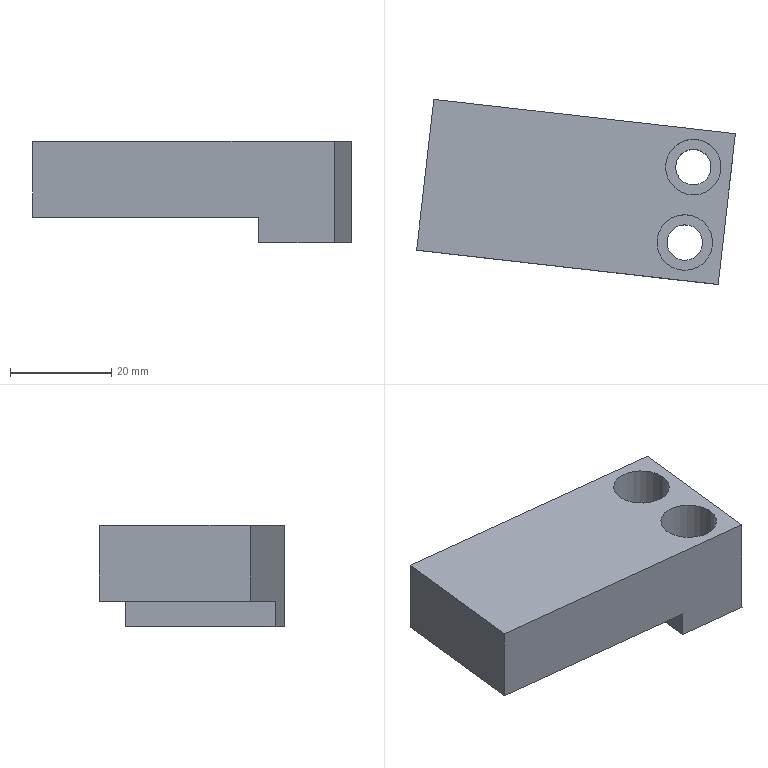Part | NX | features XQ 2 | 1 solid | 14 faces | box 63.01 x 36.599 x 20 mm | volume 26806 mm3 | plane 10 | cylinder 4 | commonest cylinder face diameters 7 x2 11 x2
STEP:
#1=CARTESIAN_POINT('',(3262.458,-294.81,-42.126));
#2=VERTEX_POINT('',#1);
#3=CARTESIAN_POINT('',(3262.458,-298.31,-42.126));
#4=DIRECTION('',(0.,0.,-1.));
#5=DIRECTION('',(0.,1.,0.));
#6=AXIS2_PLACEMENT_3D('',#3,#4,#5);
#7=CIRCLE('',#6,3.5);
#8=EDGE_CURVE('',#2,#2,#7,.T.);
#9=ORIENTED_EDGE('',*,*,#8,.T.);
#10=EDGE_LOOP('',(#9));
#11=FACE_BOUND('',#10,.T.);
#12=CARTESIAN_POINT('',(3262.458,-292.81,-42.126));
#13=VERTEX_POINT('',#12);
#14=CARTESIAN_POINT('',(3262.458,-298.31,-42.126));
#15=DIRECTION('',(0.,0.,-1.));
#16=DIRECTION('',(0.,1.,0.));
#17=AXIS2_PLACEMENT_3D('',#14,#15,#16);
#18=CIRCLE('',#17,5.5);
#19=EDGE_CURVE('',#13,#13,#18,.T.);
#20=ORIENTED_EDGE('',*,*,#19,.F.);
#21=EDGE_LOOP('',(#20));
#22=FACE_BOUND('',#21,.T.);
#23=CARTESIAN_POINT('',(3250.491,-292.921,-42.126));
#24=DIRECTION('',(0.,0.,1.));
#25=DIRECTION('',(-0.9936,0.1132,0.));
#26=AXIS2_PLACEMENT_3D('',#23,#24,#25);
#27=PLANE('',#26);
#28=ADVANCED_FACE('',(#11,#22),#27,.T.);
#29=CARTESIAN_POINT('',(3255.855,-290.009,-49.126));
#30=VERTEX_POINT('',#29);
#31=CARTESIAN_POINT('',(3252.459,-319.816,-49.126));
#32=VERTEX_POINT('',#31);
#33=CARTESIAN_POINT('',(3254.157,-304.913,-49.126));
#34=DIRECTION('',(-0.1132,-0.9936,0.));
#35=VECTOR('',#34,1000.);
#36=LINE('',#33,#35);
#37=EDGE_CURVE('',#30,#32,#36,.T.);
#38=ORIENTED_EDGE('',*,*,#37,.T.);
#39=CARTESIAN_POINT('',(3207.748,-314.722,-49.126));
#40=VERTEX_POINT('',#39);
#41=CARTESIAN_POINT('',(3247.491,-319.25,-49.126));
#42=DIRECTION('',(-0.9936,0.1132,0.));
#43=VECTOR('',#42,1000.);
#44=LINE('',#41,#43);
#45=EDGE_CURVE('',#32,#40,#44,.T.);
#46=ORIENTED_EDGE('',*,*,#45,.T.);
#47=CARTESIAN_POINT('',(3211.144,-284.915,-49.126));
#48=VERTEX_POINT('',#47);
#49=CARTESIAN_POINT('',(3197.673,-403.15,-49.126));
#50=DIRECTION('',(-0.1132,-0.9936,0.));
#51=VECTOR('',#50,1000.);
#52=LINE('',#49,#51);
#53=EDGE_CURVE('',#48,#40,#52,.T.);
#54=ORIENTED_EDGE('',*,*,#53,.F.);
#55=CARTESIAN_POINT('',(3250.887,-289.443,-49.126));
#56=DIRECTION('',(-0.9936,0.1132,0.));
#57=VECTOR('',#56,1000.);
#58=LINE('',#55,#57);
#59=EDGE_CURVE('',#30,#48,#58,.T.);
#60=ORIENTED_EDGE('',*,*,#59,.F.);
#61=EDGE_LOOP('',(#38,#46,#54,#60));
#62=FACE_BOUND('',#61,.T.);
#63=CARTESIAN_POINT('',(3250.321,-294.411,-49.126));
#64=DIRECTION('',(0.,0.,-1.));
#65=DIRECTION('',(0.9936,-0.1132,0.));
#66=AXIS2_PLACEMENT_3D('',#63,#64,#65);
#67=PLANE('',#66);
#68=ADVANCED_FACE('',(#62),#67,.T.);
#69=ORIENTED_EDGE('',*,*,#19,.T.);
#70=EDGE_LOOP('',(#69));
#71=FACE_BOUND('',#70,.T.);
#72=CARTESIAN_POINT('',(3262.458,-292.81,-34.126));
#73=VERTEX_POINT('',#72);
#74=CARTESIAN_POINT('',(3262.458,-298.31,-34.126));
#75=DIRECTION('',(0.,0.,-1.));
#76=DIRECTION('',(0.,1.,0.));
#77=AXIS2_PLACEMENT_3D('',#74,#75,#76);
#78=CIRCLE('',#77,5.5);
#79=EDGE_CURVE('',#73,#73,#78,.T.);
#80=ORIENTED_EDGE('',*,*,#79,.F.);
#81=EDGE_LOOP('',(#80));
#82=FACE_BOUND('',#81,.T.);
#83=CARTESIAN_POINT('',(3262.458,-298.31,-34.126));
#84=DIRECTION('',(0.,0.,-1.));
#85=DIRECTION('',(0.9981,0.06105,0.));
#86=AXIS2_PLACEMENT_3D('',#83,#84,#85);
#87=CYLINDRICAL_SURFACE('',#86,5.5);
#88=ADVANCED_FACE('',(#71,#82),#87,.F.);
#89=ORIENTED_EDGE('',*,*,#53,.T.);
#90=CARTESIAN_POINT('',(3207.748,-314.722,-34.126));
#91=VERTEX_POINT('',#90);
#92=CARTESIAN_POINT('',(3207.748,-314.722,-118.027));
#93=DIRECTION('',(0.,0.,1.));
#94=VECTOR('',#93,1000.);
#95=LINE('',#92,#94);
#96=EDGE_CURVE('',#40,#91,#95,.T.);
#97=ORIENTED_EDGE('',*,*,#96,.T.);
#98=CARTESIAN_POINT('',(3211.144,-284.915,-34.126));
#99=VERTEX_POINT('',#98);
#100=CARTESIAN_POINT('',(3210.578,-289.883,-34.126));
#101=DIRECTION('',(-0.1132,-0.9936,0.));
#102=VECTOR('',#101,1000.);
#103=LINE('',#100,#102);
#104=EDGE_CURVE('',#99,#91,#103,.T.);
#105=ORIENTED_EDGE('',*,*,#104,.F.);
#106=CARTESIAN_POINT('',(3211.144,-284.915,-118.027));
#107=DIRECTION('',(0.,0.,-1.));
#108=VECTOR('',#107,1000.);
#109=LINE('',#106,#108);
#110=EDGE_CURVE('',#99,#48,#109,.T.);
#111=ORIENTED_EDGE('',*,*,#110,.T.);
#112=EDGE_LOOP('',(#89,#97,#105,#111));
#113=FACE_BOUND('',#112,.T.);
#114=CARTESIAN_POINT('',(3197.673,-403.15,-118.027));
#115=DIRECTION('',(-0.9936,0.1132,0.));
#116=DIRECTION('',(0.,0.,1.));
#117=AXIS2_PLACEMENT_3D('',#114,#115,#116);
#118=PLANE('',#117);
#119=ADVANCED_FACE('',(#113),#118,.T.);
#120=ORIENTED_EDGE('',*,*,#8,.F.);
#121=EDGE_LOOP('',(#120));
#122=FACE_BOUND('',#121,.T.);
#123=CARTESIAN_POINT('',(3262.458,-301.81,-54.126));
#124=VERTEX_POINT('',#123);
#125=CARTESIAN_POINT('',(3262.458,-298.31,-54.126));
#126=DIRECTION('',(0.,0.,1.));
#127=DIRECTION('',(0.,-1.,0.));
#128=AXIS2_PLACEMENT_3D('',#125,#126,#127);
#129=CIRCLE('',#128,3.5);
#130=EDGE_CURVE('',#124,#124,#129,.T.);
#131=ORIENTED_EDGE('',*,*,#130,.F.);
#132=EDGE_LOOP('',(#131));
#133=FACE_BOUND('',#132,.T.);
#134=CARTESIAN_POINT('',(3262.458,-298.31,-34.126));
#135=DIRECTION('',(0.,0.,-1.));
#136=DIRECTION('',(0.9981,0.06105,0.));
#137=AXIS2_PLACEMENT_3D('',#134,#135,#136);
#138=CYLINDRICAL_SURFACE('',#137,3.5);
#139=ADVANCED_FACE('',(#122,#133),#138,.F.);
#140=CARTESIAN_POINT('',(3270.759,-291.707,-34.126));
#141=VERTEX_POINT('',#140);
#142=CARTESIAN_POINT('',(3267.363,-321.514,-34.126));
#143=VERTEX_POINT('',#142);
#144=CARTESIAN_POINT('',(3270.193,-296.675,-34.126));
#145=DIRECTION('',(-0.1132,-0.9936,0.));
#146=VECTOR('',#145,1000.);
#147=LINE('',#144,#146);
#148=EDGE_CURVE('',#141,#143,#147,.T.);
#149=ORIENTED_EDGE('',*,*,#148,.T.);
#150=CARTESIAN_POINT('',(3267.363,-321.514,-54.126));
#151=VERTEX_POINT('',#150);
#152=CARTESIAN_POINT('',(3267.363,-321.514,-44.126));
#153=DIRECTION('',(0.,0.,-1.));
#154=VECTOR('',#153,1000.);
#155=LINE('',#152,#154);
#156=EDGE_CURVE('',#143,#151,#155,.T.);
#157=ORIENTED_EDGE('',*,*,#156,.T.);
#158=CARTESIAN_POINT('',(3270.759,-291.707,-54.126));
#159=VERTEX_POINT('',#158);
#160=CARTESIAN_POINT('',(3270.193,-296.675,-54.126));
#161=DIRECTION('',(-0.1132,-0.9936,0.));
#162=VECTOR('',#161,1000.);
#163=LINE('',#160,#162);
#164=EDGE_CURVE('',#159,#151,#163,.T.);
#165=ORIENTED_EDGE('',*,*,#164,.F.);
#166=CARTESIAN_POINT('',(3270.759,-291.707,-44.126));
#167=DIRECTION('',(0.,0.,1.));
#168=VECTOR('',#167,1000.);
#169=LINE('',#166,#168);
#170=EDGE_CURVE('',#159,#141,#169,.T.);
#171=ORIENTED_EDGE('',*,*,#170,.T.);
#172=EDGE_LOOP('',(#149,#157,#165,#171));
#173=FACE_BOUND('',#172,.T.);
#174=CARTESIAN_POINT('',(3270.193,-296.675,-44.126));
#175=DIRECTION('',(0.9936,-0.1132,0.));
#176=DIRECTION('',(0.,0.,1.));
#177=AXIS2_PLACEMENT_3D('',#174,#175,#176);
#178=PLANE('',#177);
#179=ADVANCED_FACE('',(#173),#178,.T.);
#180=CARTESIAN_POINT('',(3255.855,-290.009,-54.126));
#181=VERTEX_POINT('',#180);
#182=CARTESIAN_POINT('',(3255.855,-290.009,-46.626));
#183=DIRECTION('',(0.,0.,-1.));
#184=VECTOR('',#183,1000.);
#185=LINE('',#182,#184);
#186=EDGE_CURVE('',#30,#181,#185,.T.);
#187=ORIENTED_EDGE('',*,*,#186,.F.);
#188=ORIENTED_EDGE('',*,*,#59,.T.);
#189=ORIENTED_EDGE('',*,*,#110,.F.);
#190=CARTESIAN_POINT('',(3250.887,-289.443,-34.126));
#191=DIRECTION('',(-0.9936,0.1132,0.));
#192=VECTOR('',#191,1000.);
#193=LINE('',#190,#192);
#194=EDGE_CURVE('',#141,#99,#193,.T.);
#195=ORIENTED_EDGE('',*,*,#194,.F.);
#196=ORIENTED_EDGE('',*,*,#170,.F.);
#197=CARTESIAN_POINT('',(3250.887,-289.443,-54.126));
#198=DIRECTION('',(0.9936,-0.1132,0.));
#199=VECTOR('',#198,1000.);
#200=LINE('',#197,#199);
#201=EDGE_CURVE('',#181,#159,#200,.T.);
#202=ORIENTED_EDGE('',*,*,#201,.F.);
#203=EDGE_LOOP('',(#187,#188,#189,#195,#196,#202));
#204=FACE_BOUND('',#203,.T.);
#205=CARTESIAN_POINT('',(3250.887,-289.443,-44.126));
#206=DIRECTION('',(0.1132,0.9936,0.));
#207=DIRECTION('',(-0.9785,0.1115,0.1736));
#208=AXIS2_PLACEMENT_3D('',#205,#206,#207);
#209=PLANE('',#208);
#210=ADVANCED_FACE('',(#204),#209,.T.);
#211=ORIENTED_EDGE('',*,*,#37,.F.);
#212=ORIENTED_EDGE('',*,*,#186,.T.);
#213=CARTESIAN_POINT('',(3252.459,-319.816,-54.126));
#214=VERTEX_POINT('',#213);
#215=CARTESIAN_POINT('',(3255.289,-294.977,-54.126));
#216=DIRECTION('',(0.1132,0.9936,0.));
#217=VECTOR('',#216,1000.);
#218=LINE('',#215,#217);
#219=EDGE_CURVE('',#214,#181,#218,.T.);
#220=ORIENTED_EDGE('',*,*,#219,.F.);
#221=CARTESIAN_POINT('',(3252.459,-319.816,-46.626));
#222=DIRECTION('',(0.,0.,1.));
#223=VECTOR('',#222,1000.);
#224=LINE('',#221,#223);
#225=EDGE_CURVE('',#214,#32,#224,.T.);
#226=ORIENTED_EDGE('',*,*,#225,.T.);
#227=EDGE_LOOP('',(#211,#212,#220,#226));
#228=FACE_BOUND('',#227,.T.);
#229=CARTESIAN_POINT('',(3254.157,-304.913,-46.626));
#230=DIRECTION('',(-0.9936,0.1132,0.));
#231=DIRECTION('',(0.,0.,-1.));
#232=AXIS2_PLACEMENT_3D('',#229,#230,#231);
#233=PLANE('',#232);
#234=ADVANCED_FACE('',(#228),#233,.T.);
#235=ORIENTED_EDGE('',*,*,#45,.F.);
#236=ORIENTED_EDGE('',*,*,#225,.F.);
#237=CARTESIAN_POINT('',(3247.491,-319.25,-54.126));
#238=DIRECTION('',(-0.9936,0.1132,0.));
#239=VECTOR('',#238,1000.);
#240=LINE('',#237,#239);
#241=EDGE_CURVE('',#151,#214,#240,.T.);
#242=ORIENTED_EDGE('',*,*,#241,.F.);
#243=ORIENTED_EDGE('',*,*,#156,.F.);
#244=CARTESIAN_POINT('',(3247.491,-319.25,-34.126));
#245=DIRECTION('',(0.9936,-0.1132,0.));
#246=VECTOR('',#245,1000.);
#247=LINE('',#244,#246);
#248=EDGE_CURVE('',#91,#143,#247,.T.);
#249=ORIENTED_EDGE('',*,*,#248,.F.);
#250=ORIENTED_EDGE('',*,*,#96,.F.);
#251=EDGE_LOOP('',(#235,#236,#242,#243,#249,#250));
#252=FACE_BOUND('',#251,.T.);
#253=CARTESIAN_POINT('',(3247.491,-319.25,-44.126));
#254=DIRECTION('',(-0.1132,-0.9936,0.));
#255=DIRECTION('',(0.9785,-0.1115,-0.1736));
#256=AXIS2_PLACEMENT_3D('',#253,#254,#255);
#257=PLANE('',#256);
#258=ADVANCED_FACE('',(#252),#257,.T.);
#259=CARTESIAN_POINT('',(3260.76,-316.714,-54.126));
#260=VERTEX_POINT('',#259);
#261=CARTESIAN_POINT('',(3260.76,-313.214,-54.126));
#262=DIRECTION('',(0.,0.,-1.));
#263=DIRECTION('',(0.,-1.,0.));
#264=AXIS2_PLACEMENT_3D('',#261,#262,#263);
#265=CIRCLE('',#264,3.5);
#266=EDGE_CURVE('',#260,#260,#265,.T.);
#267=ORIENTED_EDGE('',*,*,#266,.F.);
#268=EDGE_LOOP('',(#267));
#269=FACE_BOUND('',#268,.T.);
#270=ORIENTED_EDGE('',*,*,#241,.T.);
#271=ORIENTED_EDGE('',*,*,#219,.T.);
#272=ORIENTED_EDGE('',*,*,#201,.T.);
#273=ORIENTED_EDGE('',*,*,#164,.T.);
#274=EDGE_LOOP('',(#270,#271,#272,#273));
#275=FACE_BOUND('',#274,.T.);
#276=ORIENTED_EDGE('',*,*,#130,.T.);
#277=EDGE_LOOP('',(#276));
#278=FACE_BOUND('',#277,.T.);
#279=CARTESIAN_POINT('',(3250.321,-294.411,-54.126));
#280=DIRECTION('',(0.,0.,-1.));
#281=DIRECTION('',(0.9936,-0.1132,0.));
#282=AXIS2_PLACEMENT_3D('',#279,#280,#281);
#283=PLANE('',#282);
#284=ADVANCED_FACE('',(#269,#275,#278),#283,.T.);
#285=CARTESIAN_POINT('',(3260.76,-307.714,-34.126));
#286=VERTEX_POINT('',#285);
#287=CARTESIAN_POINT('',(3260.76,-313.214,-34.126));
#288=DIRECTION('',(0.,0.,1.));
#289=DIRECTION('',(0.,1.,0.));
#290=AXIS2_PLACEMENT_3D('',#287,#288,#289);
#291=CIRCLE('',#290,5.5);
#292=EDGE_CURVE('',#286,#286,#291,.T.);
#293=ORIENTED_EDGE('',*,*,#292,.F.);
#294=EDGE_LOOP('',(#293));
#295=FACE_BOUND('',#294,.T.);
#296=ORIENTED_EDGE('',*,*,#194,.T.);
#297=ORIENTED_EDGE('',*,*,#104,.T.);
#298=ORIENTED_EDGE('',*,*,#248,.T.);
#299=ORIENTED_EDGE('',*,*,#148,.F.);
#300=EDGE_LOOP('',(#296,#297,#298,#299));
#301=FACE_BOUND('',#300,.T.);
#302=ORIENTED_EDGE('',*,*,#79,.T.);
#303=EDGE_LOOP('',(#302));
#304=FACE_BOUND('',#303,.T.);
#305=CARTESIAN_POINT('',(3250.321,-294.411,-34.126));
#306=DIRECTION('',(0.,0.,1.));
#307=DIRECTION('',(-0.9936,0.1132,0.));
#308=AXIS2_PLACEMENT_3D('',#305,#306,#307);
#309=PLANE('',#308);
#310=ADVANCED_FACE('',(#295,#301,#304),#309,.T.);
#311=CARTESIAN_POINT('',(3260.76,-309.714,-42.126));
#312=VERTEX_POINT('',#311);
#313=CARTESIAN_POINT('',(3260.76,-313.214,-42.126));
#314=DIRECTION('',(0.,0.,-1.));
#315=DIRECTION('',(0.,1.,0.));
#316=AXIS2_PLACEMENT_3D('',#313,#314,#315);
#317=CIRCLE('',#316,3.5);
#318=EDGE_CURVE('',#312,#312,#317,.T.);
#319=ORIENTED_EDGE('',*,*,#318,.T.);
#320=EDGE_LOOP('',(#319));
#321=FACE_BOUND('',#320,.T.);
#322=CARTESIAN_POINT('',(3260.76,-307.714,-42.126));
#323=VERTEX_POINT('',#322);
#324=CARTESIAN_POINT('',(3260.76,-313.214,-42.126));
#325=DIRECTION('',(0.,0.,-1.));
#326=DIRECTION('',(0.,1.,0.));
#327=AXIS2_PLACEMENT_3D('',#324,#325,#326);
#328=CIRCLE('',#327,5.5);
#329=EDGE_CURVE('',#323,#323,#328,.T.);
#330=ORIENTED_EDGE('',*,*,#329,.F.);
#331=EDGE_LOOP('',(#330));
#332=FACE_BOUND('',#331,.T.);
#333=CARTESIAN_POINT('',(3247.887,-315.773,-42.126));
#334=DIRECTION('',(0.,0.,1.));
#335=DIRECTION('',(-0.9936,0.1132,0.));
#336=AXIS2_PLACEMENT_3D('',#333,#334,#335);
#337=PLANE('',#336);
#338=ADVANCED_FACE('',(#321,#332),#337,.T.);
#339=ORIENTED_EDGE('',*,*,#318,.F.);
#340=EDGE_LOOP('',(#339));
#341=FACE_BOUND('',#340,.T.);
#342=ORIENTED_EDGE('',*,*,#266,.T.);
#343=EDGE_LOOP('',(#342));
#344=FACE_BOUND('',#343,.T.);
#345=CARTESIAN_POINT('',(3260.76,-313.214,-34.126));
#346=DIRECTION('',(0.,0.,-1.));
#347=DIRECTION('',(0.9588,-0.284,0.));
#348=AXIS2_PLACEMENT_3D('',#345,#346,#347);
#349=CYLINDRICAL_SURFACE('',#348,3.5);
#350=ADVANCED_FACE('',(#341,#344),#349,.F.);
#351=ORIENTED_EDGE('',*,*,#329,.T.);
#352=EDGE_LOOP('',(#351));
#353=FACE_BOUND('',#352,.T.);
#354=ORIENTED_EDGE('',*,*,#292,.T.);
#355=EDGE_LOOP('',(#354));
#356=FACE_BOUND('',#355,.T.);
#357=CARTESIAN_POINT('',(3260.76,-313.214,-34.126));
#358=DIRECTION('',(0.,0.,-1.));
#359=DIRECTION('',(0.9588,-0.284,0.));
#360=AXIS2_PLACEMENT_3D('',#357,#358,#359);
#361=CYLINDRICAL_SURFACE('',#360,5.5);
#362=ADVANCED_FACE('',(#353,#356),#361,.F.);
#363=CLOSED_SHELL('',(#28,#68,#88,#119,#139,#179,#210,#234,#258,#284,#310,#338,#350,#362));
#364=MANIFOLD_SOLID_BREP('',#363);
#365=(LENGTH_UNIT()NAMED_UNIT(*)SI_UNIT(.MILLI.,.METRE.));
#366=UNCERTAINTY_MEASURE_WITH_UNIT(LENGTH_MEASURE(0.00001),#365,'','');
#367=(NAMED_UNIT(*)PLANE_ANGLE_UNIT()SI_UNIT($,.RADIAN.));
#368=(NAMED_UNIT(*)SI_UNIT($,.STERADIAN.)SOLID_ANGLE_UNIT());
#369=(GEOMETRIC_REPRESENTATION_CONTEXT(3)GLOBAL_UNCERTAINTY_ASSIGNED_CONTEXT((#366))GLOBAL_UNIT_ASSIGNED_CONTEXT((#365,#367,#368))REPRESENTATION_CONTEXT('',''));
#370=ADVANCED_BREP_SHAPE_REPRESENTATION('',(#364),#369);